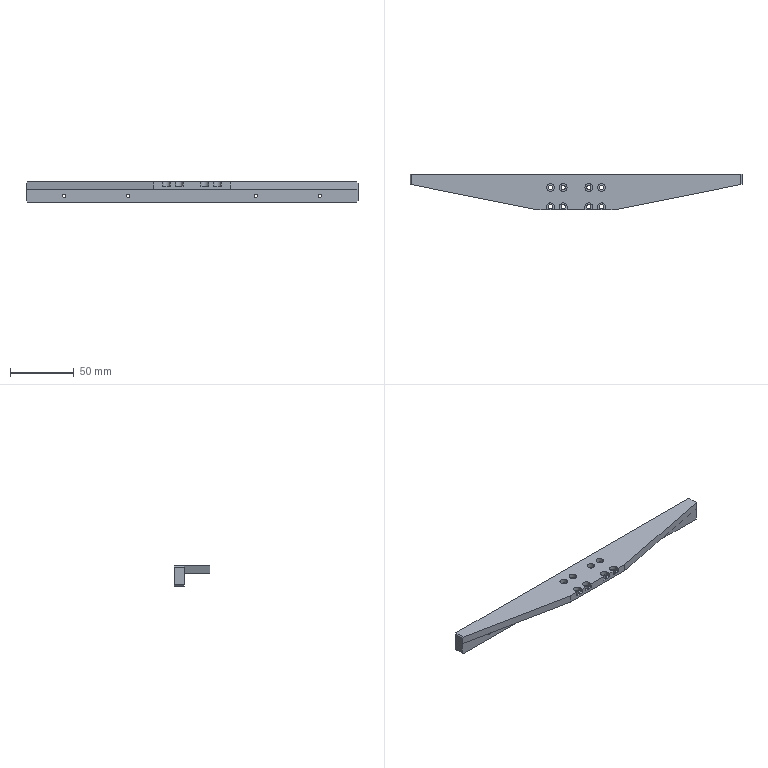Part | 1 solid | 94 faces | box 260 x 28 x 16 mm | volume 50986 mm3 | cylinder 50 | plane 30 | cone 14 | commonest cylinder face diameters 2.5 x18 3.4 x16 6 x12 4 x4